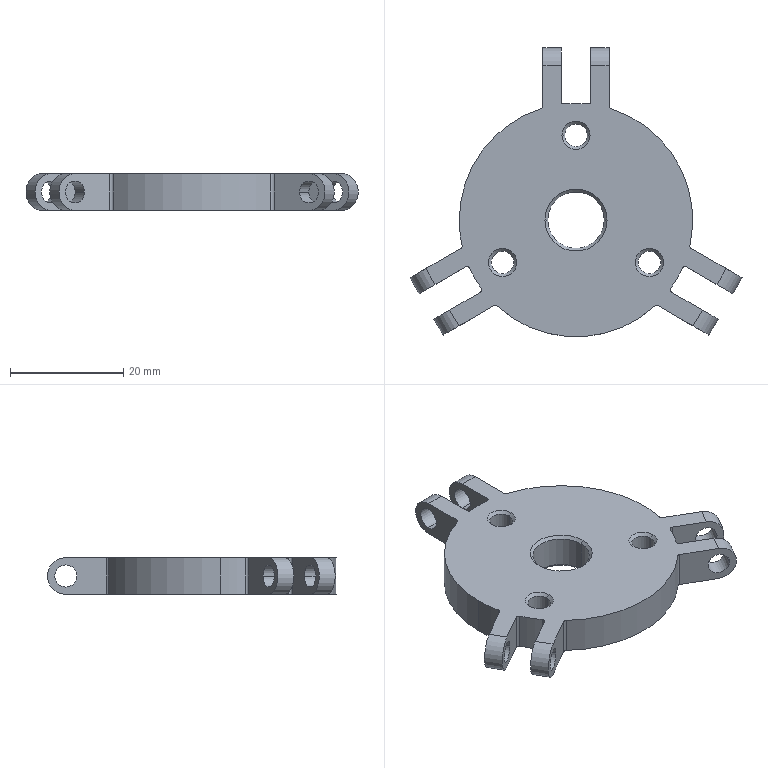Part | SolidWorks | features ICE 5, Chamfer 2, CirPattern 2, Extrusion 1, Fillet 1, Scale 1 | 1 solid | 77 faces | box 58.764 x 51.19 x 6.5 mm | volume 8922 mm3 | cylinder 47 | cone 16 | plane 14 | commonest cylinder face diameters 1 x14 3.9 x12 41.281 x7 4 x6 6.5 x6 10 x2